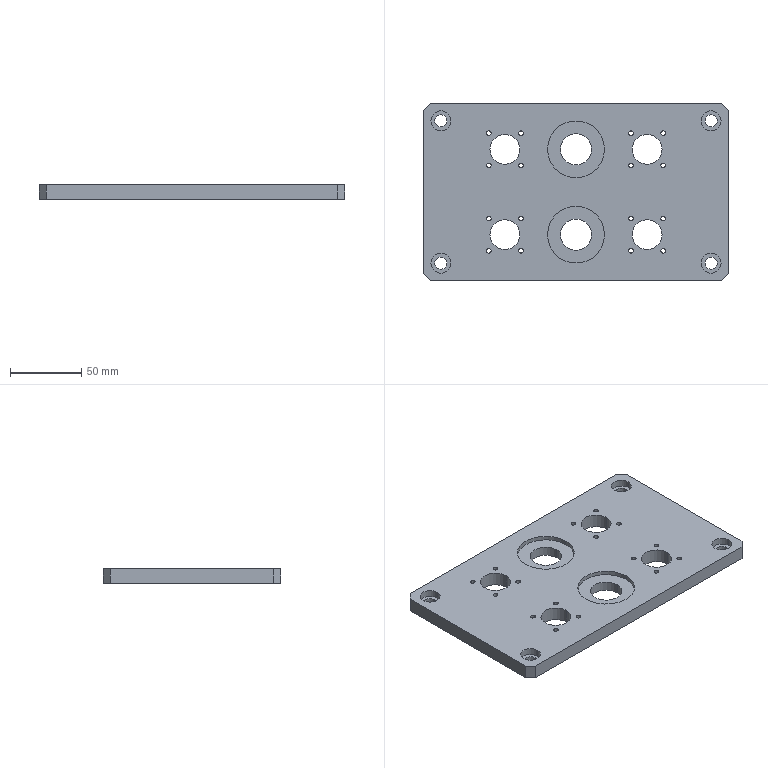Part | 1 solid | 80 faces | box 215 x 125 x 10 mm | volume 235952 mm3 | cylinder 64 | plane 16 | commonest cylinder face diameters 3.3 x32 8.5 x8 14 x8 21 x8 22 x4 40 x4